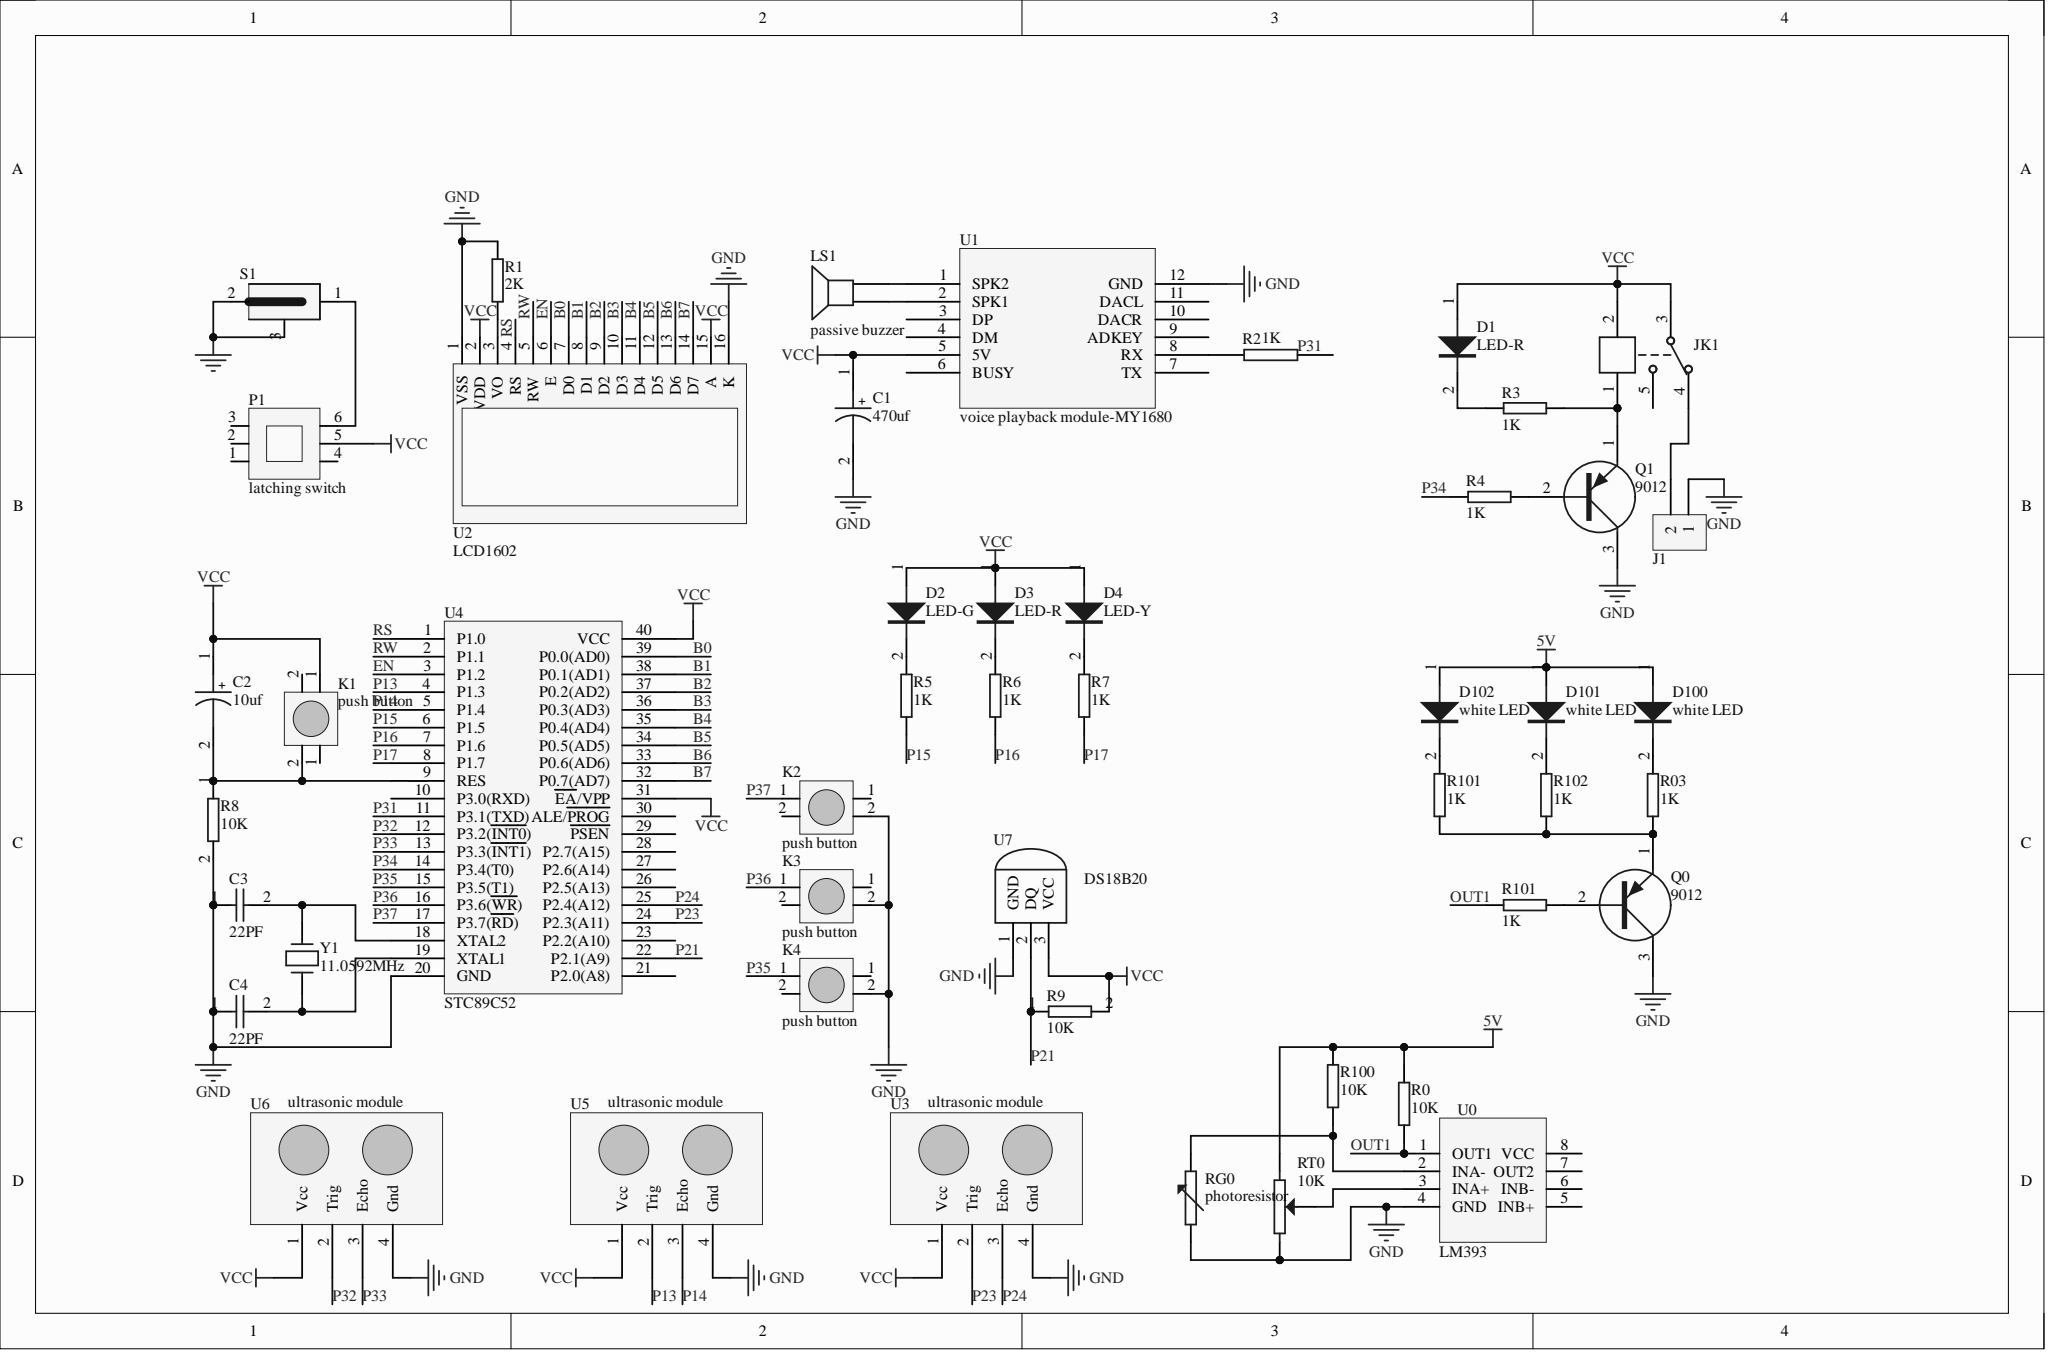Circuit board | Altium Designer | 48 parts | 51 nets
Bill of materials:
Comment,Description,Designator,Footprint,LibRef,Quantity
"470uf","","C1","RB7.6-15","电解电容","1"
"10uf","","C2","RB7.6-15","电解电容","1"
"22PF","","C3, C4","RAD-0.3","瓷片电容","2"
"LED-R","","D1, D3","LED","LED-5MM","2"
"LED-G","","D2","LED","LED-5MM","1"
"LED-Y","","D4","LED","LED-5MM","1"
"white LED","","D100, D101, D102","LED","LED-5MM","3"
"","","J1","KF301-5.0-2P","端子2P-5mm","1"
"HFKW-012-1ZW","12V one-group changeover","JK1","012-1ZW_W","HFKW-012-1ZW","1"
"push button","","K1, K2, K3, K4","四脚轻触开关","按键","4"
"passive buzzer","","LS1","PIN2","SPEAKER","1"
"latching switch","","P1","自锁开关","自锁开关","1"
"9012","","Q0, Q1","TO-92A","PNP三极管","2"
"10K","","R0, R8, R9, R100","AXIAL-0.4","电阻-定值","4"
"2K","","R1","AXIAL-0.4","电阻-定值","1"
"1K","","R2, R3, R03, R4, R5, R6, R7, R101, R102","AXIAL-0.4","","10"
"photoresistor","","RG0","AXIAL-0.6","电阻-光敏","1"
"10K","","RT0","电位器","电位器","1"
"","","S1","KLD-0202","电源接口-小","1"
"LM393","","U0","DIP-8","LM393","1"
"voice playback module-MY1680","","U1","MY1680","Component_1","1"
"LCD1602","","U2","LCD1602","LCD1602","1"
"ultrasonic module","","U3, U5, U6","HDR1X4","超声波模块","3"
"STC89C52","","U4","DIP-40","STC89C52","1"
"DS18B20","","U7","DS18B20","DS18B20","1"
"11.059MHz","","Y1","XTAL_US","晶振","1"
Netlist (Protel format):
[
C1
RB7.6-15
470uf



]
[
C2
RB7.6-15
10uf



]
[
C3
RAD-0.3
22PF



]
[
C4
RAD-0.3
22PF



]
[
D1
LED
LED-R



]
[
D2
LED
LED-G



]
[
D3
LED
LED-R



]
[
D4
LED
LED-Y



]
[
D100
LED
white LED



]
[
D101
LED
white LED



]
[
D102
LED
white LED



]
[
J1
KF301-5.0-2P




]
[
JK1
012-1ZW_W
HFKW-012-1ZW



]
[
K1
四脚轻触开关
push button



]
[
K2
四脚轻触开关
push button



]
[
K3
四脚轻触开关
push button



]
[
K4
四脚轻触开关
push button



]
[
LS1
PIN2
passive buzzer



]
[
P1
自锁开关
latching switch



]
[
Q0
TO-92A
9012



]
[
Q1
TO-92A
9012



]
[
R0
AXIAL-0.4
10K



]
[
R1
AXIAL-0.4
2K



]
[
R2
AXIAL-0.4
1K



]
[
R3
AXIAL-0.4
1K



]
[
R03
AXIAL-0.4
1K



]
[
R4
AXIAL-0.4
1K



]
[
R5
AXIAL-0.4
1K



]
[
R6
AXIAL-0.4
1K



]
[
R7
AXIAL-0.4
1K



]
[
R8
AXIAL-0.4
10K



]
[
R9
AXIAL-0.4
10K



]
[
R100
AXIAL-0.4
10K



]
[
R101
AXIAL-0.4
1K



]
[
R101
AXIAL-0.4
1K



]
[
R102
AXIAL-0.4
1K



]
[
RG0
AXIAL-0.6
photoresistor



]
[
RT0
电位器
10K



]
[
S1
KLD-0202




]
[
U0
DIP-8
LM393



]
[
U1
MY1680
voice playback module-MY1680



]
[
U2
LCD1602
LCD1602



]
[
U3
HDR1X4
ultrasonic module



]
[
U4
DIP-40
STC89C52



]
[
U5
HDR1X4
ultrasonic module



]
[
U6
HDR1X4
ultrasonic module



]
[
U7
DS18B20
DS18B20



]
[
Y1
XTAL_US
11.0592MHz



]
(
VCC
C1-1
C2-1
D1-1
D2-1
D3-1
D4-1
JK1-2
JK1-3
K1-1
P1-5
R9-2
U1-5
U2-2
U2-15
U3-1
U4-31
U4-40
U5-1
U6-1
U7-3
)
(
RW
U2-5
U4-2
)
(
RS
U2-4
U4-1
)
(
P37
K2-1
U4-17
)
(
P36
K3-1
U4-16
)
(
P35
K4-1
U4-15
)
(
P34
R4-1
U4-14
)
(
P33
U4-13
U6-3
)
(
P32
U4-12
U6-2
)
(
P24
U3-3
U4-25
)
(
P23
U3-2
U4-24
)
(
P21
R9-1
U4-22
U7-2
)
(
P17
R7-1
U4-8
)
(
P16
R6-1
U4-7
)
(
P15
R5-1
U4-6
)
(
P14
U4-5
U5-3
)
(
P13
U4-4
U5-2
)
(
OUT1
R0-1
R101-2
U0-1
)
(
NetRT0_3
RT0-3
U0-3
)
(
NetR100_1
R100-1
RG0-2
U0-2
)
(
NetR2_1
R2-1
U1-8
)
(
NetR1_1
R1-1
U2-3
)
(
NetQ1_2
Q1-2
R4-2
)
(
NetQ0_2
Q0-2
R101-1
)
(
NetQ0_1
Q0-1
R03-1
R101-1
R102-1
)
(
NetP1_6
P1-6
S1-1
)
(
NetLS1_2
LS1-2
U1-1
)
(
NetLS1_1
LS1-1
U1-2
)
(
NetJK1_1
JK1-1
Q1-1
R3-2
)
(
NetJ1_2
J1-2
JK1-4
)
(
NetD102_2
D102-2
R101-2
)
(
NetD101_2
D101-2
R102-2
)
(
NetD100_2
D100-2
R03-2
)
(
NetD4_2
D4-2
R7-2
)
(
NetD3_2
D3-2
R6-2
)
(
NetD2_2
D2-2
R5-2
)
(
NetD1_2
D1-2
R3-1
)
(
NetC4_2
C4-2
U4-19
Y1-2
)
(
NetC3_2
C3-2
U4-18
Y1-1
)
(
NetC2_2
C2-2
K1-2
R8-1
U4-9
)
(
GND
C1-2
C3-1
C4-1
J1-1
K2-2
K3-2
K4-2
Q0-3
Q1-3
R1-2
R8-2
RG0-1
RT0-2
S1-2
S1-3
U0-4
U1-12
U2-1
U2-16
U3-4
U4-20
U5-4
U6-4
U7-1
)
(
EN
U2-6
U4-3
)
(
B7
U2-14
U4-32
)
(
B6
U2-13
U4-33
)
(
B5
U2-12
U4-34
)
(
B4
U2-11
U4-35
)
(
B3
U2-10
U4-36
)
(
B2
U2-9
U4-37
)
(
B1
U2-8
U4-38
)
(
B0
U2-7
U4-39
)
(
5V
D100-1
D101-1
D102-1
R0-2
R100-2
RT0-1
)